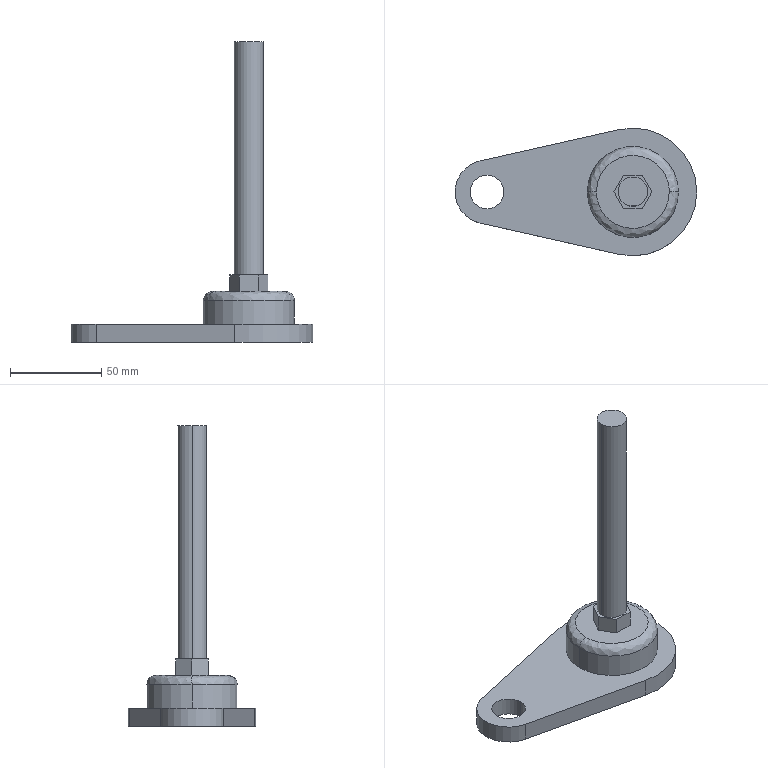Part | SolidWorks | features BaseBody 3 | 3 solids | 26 faces | box 132.5 x 70 x 165 mm | volume 127173 mm3 | plane 15 | cylinder 9 | spline 2 | commonest cylinder face diameters 16 x2 18.5 x2 50 x2 70 x2 35 x1
STEP:
#1=CARTESIAN_POINT('',(-70.75,0.,10.));
#2=VERTEX_POINT('',#1);
#3=CARTESIAN_POINT('',(-89.25,0.,10.));
#4=VERTEX_POINT('',#3);
#5=CARTESIAN_POINT('',(-80.,0.,10.));
#6=DIRECTION('',(0.,0.,-1.));
#7=DIRECTION('',(-1.,0.,0.));
#8=AXIS2_PLACEMENT_3D('',#5,#6,#7);
#9=CIRCLE('',#8,9.25);
#10=EDGE_CURVE('',#2,#4,#9,.T.);
#11=ORIENTED_EDGE('',*,*,#10,.F.);
#12=CARTESIAN_POINT('',(-70.75,0.,0.));
#13=VERTEX_POINT('',#12);
#14=CARTESIAN_POINT('',(-70.75,0.,9.9));
#15=DIRECTION('',(0.,0.,-1.));
#16=VECTOR('',#15,1000.);
#17=LINE('',#14,#16);
#18=EDGE_CURVE('',#2,#13,#17,.T.);
#19=ORIENTED_EDGE('',*,*,#18,.T.);
#20=CARTESIAN_POINT('',(-89.25,0.,0.));
#21=VERTEX_POINT('',#20);
#22=CARTESIAN_POINT('',(-80.,0.,0.));
#23=DIRECTION('',(0.,0.,-1.));
#24=DIRECTION('',(-1.,0.,0.));
#25=AXIS2_PLACEMENT_3D('',#22,#23,#24);
#26=CIRCLE('',#25,9.25);
#27=EDGE_CURVE('',#13,#21,#26,.T.);
#28=ORIENTED_EDGE('',*,*,#27,.T.);
#29=CARTESIAN_POINT('',(-89.25,0.,9.9));
#30=DIRECTION('',(0.,0.,-1.));
#31=VECTOR('',#30,1000.);
#32=LINE('',#29,#31);
#33=EDGE_CURVE('',#4,#21,#32,.T.);
#34=ORIENTED_EDGE('',*,*,#33,.F.);
#35=EDGE_LOOP('',(#11,#19,#28,#34));
#36=FACE_OUTER_BOUND('',#35,.T.);
#37=CARTESIAN_POINT('',(-80.,0.,9.9));
#38=DIRECTION('',(0.,0.,-1.));
#39=DIRECTION('',(-1.,0.,0.));
#40=AXIS2_PLACEMENT_3D('',#37,#38,#39);
#41=CYLINDRICAL_SURFACE('',#40,9.25);
#42=ADVANCED_FACE('',(#36),#41,.F.);
#43=CARTESIAN_POINT('',(-7.656,-34.152,0.));
#44=VERTEX_POINT('',#43);
#45=CARTESIAN_POINT('',(35.,0.,0.));
#46=VERTEX_POINT('',#45);
#47=CARTESIAN_POINT('',(0.,0.,0.));
#48=DIRECTION('',(0.,0.,1.));
#49=DIRECTION('',(1.,0.,0.));
#50=AXIS2_PLACEMENT_3D('',#47,#48,#49);
#51=CIRCLE('',#50,35.);
#52=EDGE_CURVE('',#44,#46,#51,.T.);
#53=ORIENTED_EDGE('',*,*,#52,.T.);
#54=CARTESIAN_POINT('',(35.,0.,10.));
#55=VERTEX_POINT('',#54);
#56=CARTESIAN_POINT('',(35.,0.,5.));
#57=DIRECTION('',(0.,0.,1.));
#58=VECTOR('',#57,1000.);
#59=LINE('',#56,#58);
#60=EDGE_CURVE('',#46,#55,#59,.T.);
#61=ORIENTED_EDGE('',*,*,#60,.T.);
#62=CARTESIAN_POINT('',(-7.656,-34.152,10.));
#63=VERTEX_POINT('',#62);
#64=CARTESIAN_POINT('',(0.,0.,10.));
#65=DIRECTION('',(0.,0.,-1.));
#66=DIRECTION('',(1.,0.,0.));
#67=AXIS2_PLACEMENT_3D('',#64,#65,#66);
#68=CIRCLE('',#67,35.);
#69=EDGE_CURVE('',#55,#63,#68,.T.);
#70=ORIENTED_EDGE('',*,*,#69,.T.);
#71=CARTESIAN_POINT('',(-7.656,-34.152,5.));
#72=DIRECTION('',(0.,0.,-1.));
#73=VECTOR('',#72,1000.);
#74=LINE('',#71,#73);
#75=EDGE_CURVE('',#63,#44,#74,.T.);
#76=ORIENTED_EDGE('',*,*,#75,.T.);
#77=EDGE_LOOP('',(#53,#61,#70,#76));
#78=FACE_OUTER_BOUND('',#77,.T.);
#79=CARTESIAN_POINT('',(0.,0.,5.));
#80=DIRECTION('',(0.,0.,1.));
#81=DIRECTION('',(1.,0.,0.));
#82=AXIS2_PLACEMENT_3D('',#79,#80,#81);
#83=CYLINDRICAL_SURFACE('',#82,35.);
#84=ADVANCED_FACE('',(#78),#83,.T.);
#85=CARTESIAN_POINT('',(-80.,0.,0.));
#86=DIRECTION('',(0.,0.,-1.));
#87=DIRECTION('',(-1.,0.,0.));
#88=AXIS2_PLACEMENT_3D('',#85,#86,#87);
#89=CIRCLE('',#88,9.25);
#90=EDGE_CURVE('',#21,#13,#89,.T.);
#91=ORIENTED_EDGE('',*,*,#90,.F.);
#92=ORIENTED_EDGE('',*,*,#27,.F.);
#93=EDGE_LOOP('',(#91,#92));
#94=FACE_BOUND('',#93,.T.);
#95=CARTESIAN_POINT('',(-83.828,17.076,0.));
#96=VERTEX_POINT('',#95);
#97=CARTESIAN_POINT('',(-83.828,-17.076,0.));
#98=VERTEX_POINT('',#97);
#99=CARTESIAN_POINT('',(-80.,0.,0.));
#100=DIRECTION('',(0.,0.,1.));
#101=DIRECTION('',(1.,0.,0.));
#102=AXIS2_PLACEMENT_3D('',#99,#100,#101);
#103=CIRCLE('',#102,17.5);
#104=EDGE_CURVE('',#96,#98,#103,.T.);
#105=ORIENTED_EDGE('',*,*,#104,.F.);
#106=CARTESIAN_POINT('',(-7.656,34.152,0.));
#107=VERTEX_POINT('',#106);
#108=CARTESIAN_POINT('',(-7.656,34.152,0.));
#109=DIRECTION('',(-0.9758,-0.2187,0.));
#110=VECTOR('',#109,1000.);
#111=LINE('',#108,#110);
#112=EDGE_CURVE('',#107,#96,#111,.T.);
#113=ORIENTED_EDGE('',*,*,#112,.F.);
#114=CARTESIAN_POINT('',(0.,0.,0.));
#115=DIRECTION('',(0.,0.,1.));
#116=DIRECTION('',(1.,0.,0.));
#117=AXIS2_PLACEMENT_3D('',#114,#115,#116);
#118=CIRCLE('',#117,35.);
#119=EDGE_CURVE('',#46,#107,#118,.T.);
#120=ORIENTED_EDGE('',*,*,#119,.F.);
#121=ORIENTED_EDGE('',*,*,#52,.F.);
#122=CARTESIAN_POINT('',(-83.828,-17.076,0.));
#123=DIRECTION('',(0.9758,-0.2187,0.));
#124=VECTOR('',#123,1000.);
#125=LINE('',#122,#124);
#126=EDGE_CURVE('',#98,#44,#125,.T.);
#127=ORIENTED_EDGE('',*,*,#126,.F.);
#128=EDGE_LOOP('',(#105,#113,#120,#121,#127));
#129=FACE_OUTER_BOUND('',#128,.T.);
#130=CARTESIAN_POINT('',(0.,0.,0.));
#131=DIRECTION('',(0.,0.,1.));
#132=DIRECTION('',(1.,0.,0.));
#133=AXIS2_PLACEMENT_3D('',#130,#131,#132);
#134=PLANE('',#133);
#135=ADVANCED_FACE('',(#94,#129),#134,.F.);
#136=ORIENTED_EDGE('',*,*,#18,.F.);
#137=CARTESIAN_POINT('',(-80.,0.,10.));
#138=DIRECTION('',(0.,0.,-1.));
#139=DIRECTION('',(-1.,0.,0.));
#140=AXIS2_PLACEMENT_3D('',#137,#138,#139);
#141=CIRCLE('',#140,9.25);
#142=EDGE_CURVE('',#4,#2,#141,.T.);
#143=ORIENTED_EDGE('',*,*,#142,.F.);
#144=ORIENTED_EDGE('',*,*,#33,.T.);
#145=ORIENTED_EDGE('',*,*,#90,.T.);
#146=EDGE_LOOP('',(#136,#143,#144,#145));
#147=FACE_OUTER_BOUND('',#146,.T.);
#148=CARTESIAN_POINT('',(-80.,0.,9.9));
#149=DIRECTION('',(0.,0.,-1.));
#150=DIRECTION('',(-1.,0.,0.));
#151=AXIS2_PLACEMENT_3D('',#148,#149,#150);
#152=CYLINDRICAL_SURFACE('',#151,9.25);
#153=ADVANCED_FACE('',(#147),#152,.F.);
#154=CARTESIAN_POINT('',(-83.828,-17.076,10.));
#155=VERTEX_POINT('',#154);
#156=CARTESIAN_POINT('',(-83.828,-17.076,5.));
#157=DIRECTION('',(0.,0.,1.));
#158=VECTOR('',#157,1000.);
#159=LINE('',#156,#158);
#160=EDGE_CURVE('',#98,#155,#159,.T.);
#161=ORIENTED_EDGE('',*,*,#160,.T.);
#162=CARTESIAN_POINT('',(-83.828,17.076,10.));
#163=VERTEX_POINT('',#162);
#164=CARTESIAN_POINT('',(-80.,0.,10.));
#165=DIRECTION('',(0.,0.,-1.));
#166=DIRECTION('',(1.,0.,0.));
#167=AXIS2_PLACEMENT_3D('',#164,#165,#166);
#168=CIRCLE('',#167,17.5);
#169=EDGE_CURVE('',#155,#163,#168,.T.);
#170=ORIENTED_EDGE('',*,*,#169,.T.);
#171=CARTESIAN_POINT('',(-83.828,17.076,5.));
#172=DIRECTION('',(0.,0.,-1.));
#173=VECTOR('',#172,1000.);
#174=LINE('',#171,#173);
#175=EDGE_CURVE('',#163,#96,#174,.T.);
#176=ORIENTED_EDGE('',*,*,#175,.T.);
#177=ORIENTED_EDGE('',*,*,#104,.T.);
#178=EDGE_LOOP('',(#161,#170,#176,#177));
#179=FACE_OUTER_BOUND('',#178,.T.);
#180=CARTESIAN_POINT('',(-80.,0.,5.));
#181=DIRECTION('',(0.,0.,1.));
#182=DIRECTION('',(1.,0.,0.));
#183=AXIS2_PLACEMENT_3D('',#180,#181,#182);
#184=CYLINDRICAL_SURFACE('',#183,17.5);
#185=ADVANCED_FACE('',(#179),#184,.T.);
#186=CARTESIAN_POINT('',(-7.656,34.152,10.));
#187=VERTEX_POINT('',#186);
#188=CARTESIAN_POINT('',(-7.656,34.152,0.));
#189=DIRECTION('',(0.,0.,1.));
#190=VECTOR('',#189,1000.);
#191=LINE('',#188,#190);
#192=EDGE_CURVE('',#107,#187,#191,.T.);
#193=ORIENTED_EDGE('',*,*,#192,.F.);
#194=ORIENTED_EDGE('',*,*,#112,.T.);
#195=ORIENTED_EDGE('',*,*,#175,.F.);
#196=CARTESIAN_POINT('',(-83.828,17.076,10.));
#197=DIRECTION('',(-0.9758,-0.2187,0.));
#198=VECTOR('',#197,1000.);
#199=LINE('',#196,#198);
#200=EDGE_CURVE('',#187,#163,#199,.T.);
#201=ORIENTED_EDGE('',*,*,#200,.F.);
#202=EDGE_LOOP('',(#193,#194,#195,#201));
#203=FACE_OUTER_BOUND('',#202,.T.);
#204=CARTESIAN_POINT('',(-83.828,17.076,0.));
#205=DIRECTION('',(0.2187,-0.9758,0.));
#206=DIRECTION('',(0.9758,0.2187,0.));
#207=AXIS2_PLACEMENT_3D('',#204,#205,#206);
#208=PLANE('',#207);
#209=ADVANCED_FACE('',(#203),#208,.F.);
#210=ORIENTED_EDGE('',*,*,#60,.F.);
#211=ORIENTED_EDGE('',*,*,#119,.T.);
#212=ORIENTED_EDGE('',*,*,#192,.T.);
#213=CARTESIAN_POINT('',(0.,0.,10.));
#214=DIRECTION('',(0.,0.,-1.));
#215=DIRECTION('',(1.,0.,0.));
#216=AXIS2_PLACEMENT_3D('',#213,#214,#215);
#217=CIRCLE('',#216,35.);
#218=EDGE_CURVE('',#187,#55,#217,.T.);
#219=ORIENTED_EDGE('',*,*,#218,.T.);
#220=EDGE_LOOP('',(#210,#211,#212,#219));
#221=FACE_OUTER_BOUND('',#220,.T.);
#222=CARTESIAN_POINT('',(0.,0.,5.));
#223=DIRECTION('',(0.,0.,1.));
#224=DIRECTION('',(1.,0.,0.));
#225=AXIS2_PLACEMENT_3D('',#222,#223,#224);
#226=CYLINDRICAL_SURFACE('',#225,35.);
#227=ADVANCED_FACE('',(#221),#226,.T.);
#228=ORIENTED_EDGE('',*,*,#160,.F.);
#229=ORIENTED_EDGE('',*,*,#126,.T.);
#230=ORIENTED_EDGE('',*,*,#75,.F.);
#231=CARTESIAN_POINT('',(-7.656,-34.152,10.));
#232=DIRECTION('',(0.9758,-0.2187,0.));
#233=VECTOR('',#232,1000.);
#234=LINE('',#231,#233);
#235=EDGE_CURVE('',#155,#63,#234,.T.);
#236=ORIENTED_EDGE('',*,*,#235,.F.);
#237=EDGE_LOOP('',(#228,#229,#230,#236));
#238=FACE_OUTER_BOUND('',#237,.T.);
#239=CARTESIAN_POINT('',(-7.656,-34.152,0.));
#240=DIRECTION('',(0.2187,0.9758,0.));
#241=DIRECTION('',(-0.9758,0.2187,0.));
#242=AXIS2_PLACEMENT_3D('',#239,#240,#241);
#243=PLANE('',#242);
#244=ADVANCED_FACE('',(#238),#243,.F.);
#245=ORIENTED_EDGE('',*,*,#142,.T.);
#246=ORIENTED_EDGE('',*,*,#10,.T.);
#247=EDGE_LOOP('',(#245,#246));
#248=FACE_BOUND('',#247,.T.);
#249=ORIENTED_EDGE('',*,*,#235,.T.);
#250=ORIENTED_EDGE('',*,*,#69,.F.);
#251=ORIENTED_EDGE('',*,*,#218,.F.);
#252=ORIENTED_EDGE('',*,*,#200,.T.);
#253=ORIENTED_EDGE('',*,*,#169,.F.);
#254=EDGE_LOOP('',(#249,#250,#251,#252,#253));
#255=FACE_OUTER_BOUND('',#254,.T.);
#256=CARTESIAN_POINT('',(0.,0.,10.));
#257=DIRECTION('',(0.,0.,1.));
#258=DIRECTION('',(1.,0.,0.));
#259=AXIS2_PLACEMENT_3D('',#256,#257,#258);
#260=PLANE('',#259);
#261=ADVANCED_FACE('',(#248,#255),#260,.T.);
#262=CLOSED_SHELL('',(#42,#84,#135,#153,#185,#209,#227,#244,#261));
#263=MANIFOLD_SOLID_BREP('',#262);
#264=CARTESIAN_POINT('',(20.,0.,28.));
#265=VERTEX_POINT('',#264);
#266=CARTESIAN_POINT('',(-20.,0.,28.));
#267=VERTEX_POINT('',#266);
#268=CARTESIAN_POINT('',(20.,0.,28.));
#269=CARTESIAN_POINT('',(20.,-40.,28.));
#270=CARTESIAN_POINT('',(-20.,-40.,28.));
#271=CARTESIAN_POINT('',(-20.,0.,28.));
#272=(BOUNDED_CURVE()B_SPLINE_CURVE(3,(#268,#269,#270,#271),.UNSPECIFIED.,.F.,.T.)B_SPLINE_CURVE_WITH_KNOTS((4,4),(0.,1.),.UNSPECIFIED.)CURVE()GEOMETRIC_REPRESENTATION_ITEM()RATIONAL_B_SPLINE_CURVE((1.,0.3333,0.3333,1.))REPRESENTATION_ITEM(''));
#273=EDGE_CURVE('',#265,#267,#272,.T.);
#274=ORIENTED_EDGE('',*,*,#273,.T.);
#275=CARTESIAN_POINT('',(-25.,0.,23.));
#276=VERTEX_POINT('',#275);
#277=CARTESIAN_POINT('',(-20.,0.,23.));
#278=DIRECTION('',(0.,-1.,0.));
#279=DIRECTION('',(-1.,0.,0.));
#280=AXIS2_PLACEMENT_3D('',#277,#278,#279);
#281=CIRCLE('',#280,5.);
#282=EDGE_CURVE('',#267,#276,#281,.T.);
#283=ORIENTED_EDGE('',*,*,#282,.T.);
#284=CARTESIAN_POINT('',(25.,0.,23.));
#285=VERTEX_POINT('',#284);
#286=CARTESIAN_POINT('',(0.,0.,23.));
#287=DIRECTION('',(0.,0.,-1.));
#288=DIRECTION('',(-1.,0.,0.));
#289=AXIS2_PLACEMENT_3D('',#286,#287,#288);
#290=CIRCLE('',#289,25.);
#291=EDGE_CURVE('',#285,#276,#290,.T.);
#292=ORIENTED_EDGE('',*,*,#291,.F.);
#293=CARTESIAN_POINT('',(20.,0.,23.));
#294=DIRECTION('',(0.,1.,0.));
#295=DIRECTION('',(1.,0.,0.));
#296=AXIS2_PLACEMENT_3D('',#293,#294,#295);
#297=CIRCLE('',#296,5.);
#298=EDGE_CURVE('',#265,#285,#297,.T.);
#299=ORIENTED_EDGE('',*,*,#298,.F.);
#300=EDGE_LOOP('',(#274,#283,#292,#299));
#301=FACE_OUTER_BOUND('',#300,.T.);
#302=CARTESIAN_POINT('',(-20.,0.,28.));
#303=CARTESIAN_POINT('',(-20.,-40.,28.));
#304=CARTESIAN_POINT('',(20.,-40.,28.));
#305=CARTESIAN_POINT('',(20.,0.,28.));
#306=CARTESIAN_POINT('',(-22.929,0.,28.));
#307=CARTESIAN_POINT('',(-22.929,-45.858,28.));
#308=CARTESIAN_POINT('',(22.929,-45.858,28.));
#309=CARTESIAN_POINT('',(22.929,0.,28.));
#310=CARTESIAN_POINT('',(-25.,0.,25.929));
#311=CARTESIAN_POINT('',(-25.,-50.,25.929));
#312=CARTESIAN_POINT('',(25.,-50.,25.929));
#313=CARTESIAN_POINT('',(25.,0.,25.929));
#314=CARTESIAN_POINT('',(-25.,0.,23.));
#315=CARTESIAN_POINT('',(-25.,-50.,23.));
#316=CARTESIAN_POINT('',(25.,-50.,23.));
#317=CARTESIAN_POINT('',(25.,0.,23.));
#318=(BOUNDED_SURFACE()B_SPLINE_SURFACE(3,3,((#302,#303,#304,#305),(#306,#307,#308,#309),(#310,#311,#312,#313),(#314,#315,#316,#317)),.UNSPECIFIED.,.F.,.F.,.F.)B_SPLINE_SURFACE_WITH_KNOTS((4,4),(4,4),(0.,1.),(0.,1.),.UNSPECIFIED.)GEOMETRIC_REPRESENTATION_ITEM()RATIONAL_B_SPLINE_SURFACE(((1.,0.3333,0.3333,1.),(0.8047,0.2682,0.2682,0.8047),(0.8047,0.2682,0.2682,0.8047),(1.,0.3333,0.3333,1.)))REPRESENTATION_ITEM('')SURFACE());
#319=ADVANCED_FACE('',(#301),#318,.T.);
#320=CARTESIAN_POINT('',(0.,0.,23.));
#321=DIRECTION('',(0.,0.,-1.));
#322=DIRECTION('',(-1.,0.,0.));
#323=AXIS2_PLACEMENT_3D('',#320,#321,#322);
#324=CIRCLE('',#323,25.);
#325=EDGE_CURVE('',#276,#285,#324,.T.);
#326=ORIENTED_EDGE('',*,*,#325,.T.);
#327=CARTESIAN_POINT('',(25.,0.,10.));
#328=VERTEX_POINT('',#327);
#329=CARTESIAN_POINT('',(25.,0.,28.));
#330=DIRECTION('',(0.,0.,-1.));
#331=VECTOR('',#330,1000.);
#332=LINE('',#329,#331);
#333=EDGE_CURVE('',#285,#328,#332,.T.);
#334=ORIENTED_EDGE('',*,*,#333,.T.);
#335=CARTESIAN_POINT('',(-25.,0.,10.));
#336=VERTEX_POINT('',#335);
#337=CARTESIAN_POINT('',(0.,0.,10.));
#338=DIRECTION('',(0.,0.,1.));
#339=DIRECTION('',(-1.,0.,0.));
#340=AXIS2_PLACEMENT_3D('',#337,#338,#339);
#341=CIRCLE('',#340,25.);
#342=EDGE_CURVE('',#328,#336,#341,.T.);
#343=ORIENTED_EDGE('',*,*,#342,.T.);
#344=CARTESIAN_POINT('',(-25.,0.,28.));
#345=DIRECTION('',(0.,0.,-1.));
#346=VECTOR('',#345,1000.);
#347=LINE('',#344,#346);
#348=EDGE_CURVE('',#276,#336,#347,.T.);
#349=ORIENTED_EDGE('',*,*,#348,.F.);
#350=EDGE_LOOP('',(#326,#334,#343,#349));
#351=FACE_OUTER_BOUND('',#350,.T.);
#352=CARTESIAN_POINT('',(0.,0.,28.));
#353=DIRECTION('',(0.,0.,-1.));
#354=DIRECTION('',(-1.,0.,0.));
#355=AXIS2_PLACEMENT_3D('',#352,#353,#354);
#356=CYLINDRICAL_SURFACE('',#355,25.);
#357=ADVANCED_FACE('',(#351),#356,.T.);
#358=CARTESIAN_POINT('',(0.,0.,10.));
#359=DIRECTION('',(0.,0.,1.));
#360=DIRECTION('',(-1.,0.,0.));
#361=AXIS2_PLACEMENT_3D('',#358,#359,#360);
#362=CIRCLE('',#361,25.);
#363=EDGE_CURVE('',#336,#328,#362,.T.);
#364=ORIENTED_EDGE('',*,*,#363,.F.);
#365=ORIENTED_EDGE('',*,*,#342,.F.);
#366=EDGE_LOOP('',(#364,#365));
#367=FACE_OUTER_BOUND('',#366,.T.);
#368=CARTESIAN_POINT('',(-87.5,0.,10.));
#369=DIRECTION('',(0.,0.,1.));
#370=DIRECTION('',(1.,0.,0.));
#371=AXIS2_PLACEMENT_3D('',#368,#369,#370);
#372=PLANE('',#371);
#373=ADVANCED_FACE('',(#367),#372,.F.);
#374=ORIENTED_EDGE('',*,*,#333,.F.);
#375=ORIENTED_EDGE('',*,*,#291,.T.);
#376=ORIENTED_EDGE('',*,*,#348,.T.);
#377=ORIENTED_EDGE('',*,*,#363,.T.);
#378=EDGE_LOOP('',(#374,#375,#376,#377));
#379=FACE_OUTER_BOUND('',#378,.T.);
#380=CARTESIAN_POINT('',(0.,0.,28.));
#381=DIRECTION('',(0.,0.,-1.));
#382=DIRECTION('',(-1.,0.,0.));
#383=AXIS2_PLACEMENT_3D('',#380,#381,#382);
#384=CYLINDRICAL_SURFACE('',#383,25.);
#385=ADVANCED_FACE('',(#379),#384,.T.);
#386=ORIENTED_EDGE('',*,*,#282,.F.);
#387=CARTESIAN_POINT('',(-20.,0.,28.));
#388=CARTESIAN_POINT('',(-20.,40.,28.));
#389=CARTESIAN_POINT('',(20.,40.,28.));
#390=CARTESIAN_POINT('',(20.,0.,28.));
#391=(BOUNDED_CURVE()B_SPLINE_CURVE(3,(#387,#388,#389,#390),.UNSPECIFIED.,.F.,.F.)B_SPLINE_CURVE_WITH_KNOTS((4,4),(0.,1.),.UNSPECIFIED.)CURVE()GEOMETRIC_REPRESENTATION_ITEM()RATIONAL_B_SPLINE_CURVE((1.,0.3333,0.3333,1.))REPRESENTATION_ITEM(''));
#392=EDGE_CURVE('',#267,#265,#391,.T.);
#393=ORIENTED_EDGE('',*,*,#392,.T.);
#394=ORIENTED_EDGE('',*,*,#298,.T.);
#395=ORIENTED_EDGE('',*,*,#325,.F.);
#396=EDGE_LOOP('',(#386,#393,#394,#395));
#397=FACE_OUTER_BOUND('',#396,.T.);
#398=CARTESIAN_POINT('',(20.,0.,28.));
#399=CARTESIAN_POINT('',(20.,40.,28.));
#400=CARTESIAN_POINT('',(-20.,40.,28.));
#401=CARTESIAN_POINT('',(-20.,0.,28.));
#402=CARTESIAN_POINT('',(22.929,0.,28.));
#403=CARTESIAN_POINT('',(22.929,45.858,28.));
#404=CARTESIAN_POINT('',(-22.929,45.858,28.));
#405=CARTESIAN_POINT('',(-22.929,0.,28.));
#406=CARTESIAN_POINT('',(25.,0.,25.929));
#407=CARTESIAN_POINT('',(25.,50.,25.929));
#408=CARTESIAN_POINT('',(-25.,50.,25.929));
#409=CARTESIAN_POINT('',(-25.,0.,25.929));
#410=CARTESIAN_POINT('',(25.,0.,23.));
#411=CARTESIAN_POINT('',(25.,50.,23.));
#412=CARTESIAN_POINT('',(-25.,50.,23.));
#413=CARTESIAN_POINT('',(-25.,0.,23.));
#414=(BOUNDED_SURFACE()B_SPLINE_SURFACE(3,3,((#398,#399,#400,#401),(#402,#403,#404,#405),(#406,#407,#408,#409),(#410,#411,#412,#413)),.UNSPECIFIED.,.F.,.F.,.F.)B_SPLINE_SURFACE_WITH_KNOTS((4,4),(4,4),(0.,1.),(0.,1.),.UNSPECIFIED.)GEOMETRIC_REPRESENTATION_ITEM()RATIONAL_B_SPLINE_SURFACE(((1.,0.3333,0.3333,1.),(0.8047,0.2682,0.2682,0.8047),(0.8047,0.2682,0.2682,0.8047),(1.,0.3333,0.3333,1.)))REPRESENTATION_ITEM('')SURFACE());
#415=ADVANCED_FACE('',(#397),#414,.T.);
#416=ORIENTED_EDGE('',*,*,#273,.F.);
#417=ORIENTED_EDGE('',*,*,#392,.F.);
#418=EDGE_LOOP('',(#416,#417));
#419=FACE_OUTER_BOUND('',#418,.T.);
#420=CARTESIAN_POINT('',(0.,0.,28.));
#421=DIRECTION('',(0.,0.,1.));
#422=DIRECTION('',(1.,0.,0.));
#423=AXIS2_PLACEMENT_3D('',#420,#421,#422);
#424=PLANE('',#423);
#425=ADVANCED_FACE('',(#419),#424,.T.);
#426=CLOSED_SHELL('',(#319,#357,#373,#385,#415,#425));
#427=MANIFOLD_SOLID_BREP('',#426);
#428=CARTESIAN_POINT('',(8.,0.,165.));
#429=VERTEX_POINT('',#428);
#430=CARTESIAN_POINT('',(-8.,0.,165.));
#431=VERTEX_POINT('',#430);
#432=CARTESIAN_POINT('',(0.,0.,165.));
#433=DIRECTION('',(0.,0.,1.));
#434=DIRECTION('',(1.,0.,0.));
#435=AXIS2_PLACEMENT_3D('',#432,#433,#434);
#436=CIRCLE('',#435,8.);
#437=EDGE_CURVE('',#429,#431,#436,.T.);
#438=ORIENTED_EDGE('',*,*,#437,.F.);
#439=CARTESIAN_POINT('',(8.,0.,37.));
#440=VERTEX_POINT('',#439);
#441=CARTESIAN_POINT('',(8.,0.,165.));
#442=DIRECTION('',(0.,0.,-1.));
#443=VECTOR('',#442,1000.);
#444=LINE('',#441,#443);
#445=EDGE_CURVE('',#429,#440,#444,.T.);
#446=ORIENTED_EDGE('',*,*,#445,.T.);
#447=CARTESIAN_POINT('',(-8.,0.,37.));
#448=VERTEX_POINT('',#447);
#449=CARTESIAN_POINT('',(0.,0.,37.));
#450=DIRECTION('',(0.,0.,1.));
#451=DIRECTION('',(1.,0.,0.));
#452=AXIS2_PLACEMENT_3D('',#449,#450,#451);
#453=CIRCLE('',#452,8.);
#454=EDGE_CURVE('',#440,#448,#453,.T.);
#455=ORIENTED_EDGE('',*,*,#454,.T.);
#456=CARTESIAN_POINT('',(-8.,0.,165.));
#457=DIRECTION('',(0.,0.,-1.));
#458=VECTOR('',#457,1000.);
#459=LINE('',#456,#458);
#460=EDGE_CURVE('',#431,#448,#459,.T.);
#461=ORIENTED_EDGE('',*,*,#460,.F.);
#462=EDGE_LOOP('',(#438,#446,#455,#461));
#463=FACE_OUTER_BOUND('',#462,.T.);
#464=CARTESIAN_POINT('',(0.,0.,165.));
#465=DIRECTION('',(0.,0.,-1.));
#466=DIRECTION('',(-1.,0.,0.));
#467=AXIS2_PLACEMENT_3D('',#464,#465,#466);
#468=CYLINDRICAL_SURFACE('',#467,8.);
#469=ADVANCED_FACE('',(#463),#468,.T.);
#470=ORIENTED_EDGE('',*,*,#445,.F.);
#471=CARTESIAN_POINT('',(0.,0.,165.));
#472=DIRECTION('',(0.,0.,1.));
#473=DIRECTION('',(1.,0.,0.));
#474=AXIS2_PLACEMENT_3D('',#471,#472,#473);
#475=CIRCLE('',#474,8.);
#476=EDGE_CURVE('',#431,#429,#475,.T.);
#477=ORIENTED_EDGE('',*,*,#476,.F.);
#478=ORIENTED_EDGE('',*,*,#460,.T.);
#479=CARTESIAN_POINT('',(0.,0.,37.));
#480=DIRECTION('',(0.,0.,1.));
#481=DIRECTION('',(1.,0.,0.));
#482=AXIS2_PLACEMENT_3D('',#479,#480,#481);
#483=CIRCLE('',#482,8.);
#484=EDGE_CURVE('',#448,#440,#483,.T.);
#485=ORIENTED_EDGE('',*,*,#484,.T.);
#486=EDGE_LOOP('',(#470,#477,#478,#485));
#487=FACE_OUTER_BOUND('',#486,.T.);
#488=CARTESIAN_POINT('',(0.,0.,165.));
#489=DIRECTION('',(0.,0.,-1.));
#490=DIRECTION('',(-1.,0.,0.));
#491=AXIS2_PLACEMENT_3D('',#488,#489,#490);
#492=CYLINDRICAL_SURFACE('',#491,8.);
#493=ADVANCED_FACE('',(#487),#492,.T.);
#494=ORIENTED_EDGE('',*,*,#476,.T.);
#495=ORIENTED_EDGE('',*,*,#437,.T.);
#496=EDGE_LOOP('',(#494,#495));
#497=FACE_OUTER_BOUND('',#496,.T.);
#498=CARTESIAN_POINT('',(0.,0.,165.));
#499=DIRECTION('',(0.,0.,1.));
#500=DIRECTION('',(1.,0.,0.));
#501=AXIS2_PLACEMENT_3D('',#498,#499,#500);
#502=PLANE('',#501);
#503=ADVANCED_FACE('',(#497),#502,.T.);
#504=CARTESIAN_POINT('',(5.196,9.,37.));
#505=VERTEX_POINT('',#504);
#506=CARTESIAN_POINT('',(-5.196,9.,37.));
#507=VERTEX_POINT('',#506);
#508=CARTESIAN_POINT('',(0.,9.,37.));
#509=DIRECTION('',(-1.,0.,0.));
#510=VECTOR('',#509,1000.);
#511=LINE('',#508,#510);
#512=EDGE_CURVE('',#505,#507,#511,.T.);
#513=ORIENTED_EDGE('',*,*,#512,.T.);
#514=CARTESIAN_POINT('',(-10.392,0.,37.));
#515=VERTEX_POINT('',#514);
#516=CARTESIAN_POINT('',(-5.196,9.,37.));
#517=DIRECTION('',(-0.5,-0.866,0.));
#518=VECTOR('',#517,1000.);
#519=LINE('',#516,#518);
#520=EDGE_CURVE('',#507,#515,#519,.T.);
#521=ORIENTED_EDGE('',*,*,#520,.T.);
#522=CARTESIAN_POINT('',(-5.196,-9.,37.));
#523=VERTEX_POINT('',#522);
#524=CARTESIAN_POINT('',(-10.392,0.,37.));
#525=DIRECTION('',(0.5,-0.866,0.));
#526=VECTOR('',#525,1000.);
#527=LINE('',#524,#526);
#528=EDGE_CURVE('',#515,#523,#527,.T.);
#529=ORIENTED_EDGE('',*,*,#528,.T.);
#530=CARTESIAN_POINT('',(5.196,-9.,37.));
#531=VERTEX_POINT('',#530);
#532=CARTESIAN_POINT('',(0.,-9.,37.));
#533=DIRECTION('',(1.,0.,0.));
#534=VECTOR('',#533,1000.);
#535=LINE('',#532,#534);
#536=EDGE_CURVE('',#523,#531,#535,.T.);
#537=ORIENTED_EDGE('',*,*,#536,.T.);
#538=CARTESIAN_POINT('',(10.392,0.,37.));
#539=VERTEX_POINT('',#538);
#540=CARTESIAN_POINT('',(5.196,-9.,37.));
#541=DIRECTION('',(0.5,0.866,0.));
#542=VECTOR('',#541,1000.);
#543=LINE('',#540,#542);
#544=EDGE_CURVE('',#531,#539,#543,.T.);
#545=ORIENTED_EDGE('',*,*,#544,.T.);
#546=CARTESIAN_POINT('',(10.392,0.,37.));
#547=DIRECTION('',(-0.5,0.866,0.));
#548=VECTOR('',#547,1000.);
#549=LINE('',#546,#548);
#550=EDGE_CURVE('',#539,#505,#549,.T.);
#551=ORIENTED_EDGE('',*,*,#550,.T.);
#552=EDGE_LOOP('',(#513,#521,#529,#537,#545,#551));
#553=FACE_OUTER_BOUND('',#552,.T.);
#554=ORIENTED_EDGE('',*,*,#484,.F.);
#555=ORIENTED_EDGE('',*,*,#454,.F.);
#556=EDGE_LOOP('',(#554,#555));
#557=FACE_BOUND('',#556,.T.);
#558=CARTESIAN_POINT('',(0.,0.,37.));
#559=DIRECTION('',(0.,0.,1.));
#560=DIRECTION('',(1.,0.,0.));
#561=AXIS2_PLACEMENT_3D('',#558,#559,#560);
#562=PLANE('',#561);
#563=ADVANCED_FACE('',(#553,#557),#562,.T.);
#564=CARTESIAN_POINT('',(-5.196,9.,28.));
#565=VERTEX_POINT('',#564);
#566=CARTESIAN_POINT('',(-10.392,0.,28.));
#567=VERTEX_POINT('',#566);
#568=CARTESIAN_POINT('',(-5.196,9.,28.));
#569=DIRECTION('',(-0.5,-0.866,0.));
#570=VECTOR('',#569,1000.);
#571=LINE('',#568,#570);
#572=EDGE_CURVE('',#565,#567,#571,.T.);
#573=ORIENTED_EDGE('',*,*,#572,.T.);
#574=CARTESIAN_POINT('',(-10.392,0.,28.));
#575=DIRECTION('',(0.,0.,1.));
#576=VECTOR('',#575,1000.);
#577=LINE('',#574,#576);
#578=EDGE_CURVE('',#567,#515,#577,.T.);
#579=ORIENTED_EDGE('',*,*,#578,.T.);
#580=ORIENTED_EDGE('',*,*,#520,.F.);
#581=CARTESIAN_POINT('',(-5.196,9.,28.));
#582=DIRECTION('',(0.,0.,-1.));
#583=VECTOR('',#582,1000.);
#584=LINE('',#581,#583);
#585=EDGE_CURVE('',#507,#565,#584,.T.);
#586=ORIENTED_EDGE('',*,*,#585,.T.);
#587=EDGE_LOOP('',(#573,#579,#580,#586));
#588=FACE_OUTER_BOUND('',#587,.T.);
#589=CARTESIAN_POINT('',(-5.196,9.,28.));
#590=DIRECTION('',(-0.866,0.5,0.));
#591=DIRECTION('',(-0.5,-0.866,0.));
#592=AXIS2_PLACEMENT_3D('',#589,#590,#591);
#593=PLANE('',#592);
#594=ADVANCED_FACE('',(#588),#593,.T.);
#595=CARTESIAN_POINT('',(5.196,9.,28.));
#596=VERTEX_POINT('',#595);
#597=CARTESIAN_POINT('',(5.196,9.,28.));
#598=DIRECTION('',(-1.,0.,0.));
#599=VECTOR('',#598,1000.);
#600=LINE('',#597,#599);
#601=EDGE_CURVE('',#596,#565,#600,.T.);
#602=ORIENTED_EDGE('',*,*,#601,.T.);
#603=ORIENTED_EDGE('',*,*,#585,.F.);
#604=ORIENTED_EDGE('',*,*,#512,.F.);
#605=CARTESIAN_POINT('',(5.196,9.,28.));
#606=DIRECTION('',(0.,0.,-1.));
#607=VECTOR('',#606,1000.);
#608=LINE('',#605,#607);
#609=EDGE_CURVE('',#505,#596,#608,.T.);
#610=ORIENTED_EDGE('',*,*,#609,.T.);
#611=EDGE_LOOP('',(#602,#603,#604,#610));
#612=FACE_OUTER_BOUND('',#611,.T.);
#613=CARTESIAN_POINT('',(5.196,9.,28.));
#614=DIRECTION('',(0.,1.,0.));
#615=DIRECTION('',(-1.,0.,0.));
#616=AXIS2_PLACEMENT_3D('',#613,#614,#615);
#617=PLANE('',#616);
#618=ADVANCED_FACE('',(#612),#617,.T.);
#619=CARTESIAN_POINT('',(10.392,0.,28.));
#620=VERTEX_POINT('',#619);
#621=CARTESIAN_POINT('',(10.392,0.,28.));
#622=DIRECTION('',(-0.5,0.866,0.));
#623=VECTOR('',#622,1000.);
#624=LINE('',#621,#623);
#625=EDGE_CURVE('',#620,#596,#624,.T.);
#626=ORIENTED_EDGE('',*,*,#625,.T.);
#627=ORIENTED_EDGE('',*,*,#609,.F.);
#628=ORIENTED_EDGE('',*,*,#550,.F.);
#629=CARTESIAN_POINT('',(10.392,0.,28.));
#630=DIRECTION('',(0.,0.,-1.));
#631=VECTOR('',#630,1000.);
#632=LINE('',#629,#631);
#633=EDGE_CURVE('',#539,#620,#632,.T.);
#634=ORIENTED_EDGE('',*,*,#633,.T.);
#635=EDGE_LOOP('',(#626,#627,#628,#634));
#636=FACE_OUTER_BOUND('',#635,.T.);
#637=CARTESIAN_POINT('',(10.392,0.,28.));
#638=DIRECTION('',(0.866,0.5,0.));
#639=DIRECTION('',(-0.5,0.866,0.));
#640=AXIS2_PLACEMENT_3D('',#637,#638,#639);
#641=PLANE('',#640);
#642=ADVANCED_FACE('',(#636),#641,.T.);
#643=CARTESIAN_POINT('',(5.196,-9.,28.));
#644=VERTEX_POINT('',#643);
#645=CARTESIAN_POINT('',(5.196,-9.,28.));
#646=DIRECTION('',(0.5,0.866,0.));
#647=VECTOR('',#646,1000.);
#648=LINE('',#645,#647);
#649=EDGE_CURVE('',#644,#620,#648,.T.);
#650=ORIENTED_EDGE('',*,*,#649,.T.);
#651=ORIENTED_EDGE('',*,*,#633,.F.);
#652=ORIENTED_EDGE('',*,*,#544,.F.);
#653=CARTESIAN_POINT('',(5.196,-9.,28.));
#654=DIRECTION('',(0.,0.,-1.));
#655=VECTOR('',#654,1000.);
#656=LINE('',#653,#655);
#657=EDGE_CURVE('',#531,#644,#656,.T.);
#658=ORIENTED_EDGE('',*,*,#657,.T.);
#659=EDGE_LOOP('',(#650,#651,#652,#658));
#660=FACE_OUTER_BOUND('',#659,.T.);
#661=CARTESIAN_POINT('',(5.196,-9.,28.));
#662=DIRECTION('',(0.866,-0.5,0.));
#663=DIRECTION('',(0.5,0.866,0.));
#664=AXIS2_PLACEMENT_3D('',#661,#662,#663);
#665=PLANE('',#664);
#666=ADVANCED_FACE('',(#660),#665,.T.);
#667=CARTESIAN_POINT('',(-5.196,-9.,28.));
#668=VERTEX_POINT('',#667);
#669=CARTESIAN_POINT('',(-5.196,-9.,28.));
#670=DIRECTION('',(1.,0.,0.));
#671=VECTOR('',#670,1000.);
#672=LINE('',#669,#671);
#673=EDGE_CURVE('',#668,#644,#672,.T.);
#674=ORIENTED_EDGE('',*,*,#673,.T.);
#675=ORIENTED_EDGE('',*,*,#657,.F.);
#676=ORIENTED_EDGE('',*,*,#536,.F.);
#677=CARTESIAN_POINT('',(-5.196,-9.,28.));
#678=DIRECTION('',(0.,0.,-1.));
#679=VECTOR('',#678,1000.);
#680=LINE('',#677,#679);
#681=EDGE_CURVE('',#523,#668,#680,.T.);
#682=ORIENTED_EDGE('',*,*,#681,.T.);
#683=EDGE_LOOP('',(#674,#675,#676,#682));
#684=FACE_OUTER_BOUND('',#683,.T.);
#685=CARTESIAN_POINT('',(-5.196,-9.,28.));
#686=DIRECTION('',(0.,-1.,0.));
#687=DIRECTION('',(0.,0.,-1.));
#688=AXIS2_PLACEMENT_3D('',#685,#686,#687);
#689=PLANE('',#688);
#690=ADVANCED_FACE('',(#684),#689,.T.);
#691=CARTESIAN_POINT('',(-10.392,0.,28.));
#692=DIRECTION('',(0.5,-0.866,0.));
#693=VECTOR('',#692,1000.);
#694=LINE('',#691,#693);
#695=EDGE_CURVE('',#567,#668,#694,.T.);
#696=ORIENTED_EDGE('',*,*,#695,.T.);
#697=ORIENTED_EDGE('',*,*,#681,.F.);
#698=ORIENTED_EDGE('',*,*,#528,.F.);
#699=ORIENTED_EDGE('',*,*,#578,.F.);
#700=EDGE_LOOP('',(#696,#697,#698,#699));
#701=FACE_OUTER_BOUND('',#700,.T.);
#702=CARTESIAN_POINT('',(-10.392,0.,28.));
#703=DIRECTION('',(-0.866,-0.5,0.));
#704=DIRECTION('',(0.5,-0.866,0.));
#705=AXIS2_PLACEMENT_3D('',#702,#703,#704);
#706=PLANE('',#705);
#707=ADVANCED_FACE('',(#701),#706,.T.);
#708=ORIENTED_EDGE('',*,*,#695,.F.);
#709=ORIENTED_EDGE('',*,*,#572,.F.);
#710=ORIENTED_EDGE('',*,*,#601,.F.);
#711=ORIENTED_EDGE('',*,*,#625,.F.);
#712=ORIENTED_EDGE('',*,*,#649,.F.);
#713=ORIENTED_EDGE('',*,*,#673,.F.);
#714=EDGE_LOOP('',(#708,#709,#710,#711,#712,#713));
#715=FACE_OUTER_BOUND('',#714,.T.);
#716=CARTESIAN_POINT('',(0.,0.,28.));
#717=DIRECTION('',(0.,0.,1.));
#718=DIRECTION('',(1.,0.,0.));
#719=AXIS2_PLACEMENT_3D('',#716,#717,#718);
#720=PLANE('',#719);
#721=ADVANCED_FACE('',(#715),#720,.F.);
#722=CLOSED_SHELL('',(#469,#493,#503,#563,#594,#618,#642,#666,#690,#707,#721));
#723=MANIFOLD_SOLID_BREP('',#722);
#724=CARTESIAN_POINT('',(0.,0.,0.));
#725=DIRECTION('',(0.,0.,1.));
#726=DIRECTION('',(1.,0.,0.));
#727=AXIS2_PLACEMENT_3D('',#724,#725,#726);
#728=(LENGTH_UNIT()NAMED_UNIT(*)SI_UNIT(.MILLI.,.METRE.));
#729=UNCERTAINTY_MEASURE_WITH_UNIT(LENGTH_MEASURE(0.00001),#728,'','');
#730=(NAMED_UNIT(*)PLANE_ANGLE_UNIT()SI_UNIT($,.RADIAN.));
#731=(NAMED_UNIT(*)SI_UNIT($,.STERADIAN.)SOLID_ANGLE_UNIT());
#732=(GEOMETRIC_REPRESENTATION_CONTEXT(3)GLOBAL_UNCERTAINTY_ASSIGNED_CONTEXT((#729))GLOBAL_UNIT_ASSIGNED_CONTEXT((#728,#730,#731))REPRESENTATION_CONTEXT('',''));
#733=ADVANCED_BREP_SHAPE_REPRESENTATION('',(#263,#427,#723,#727),#732);